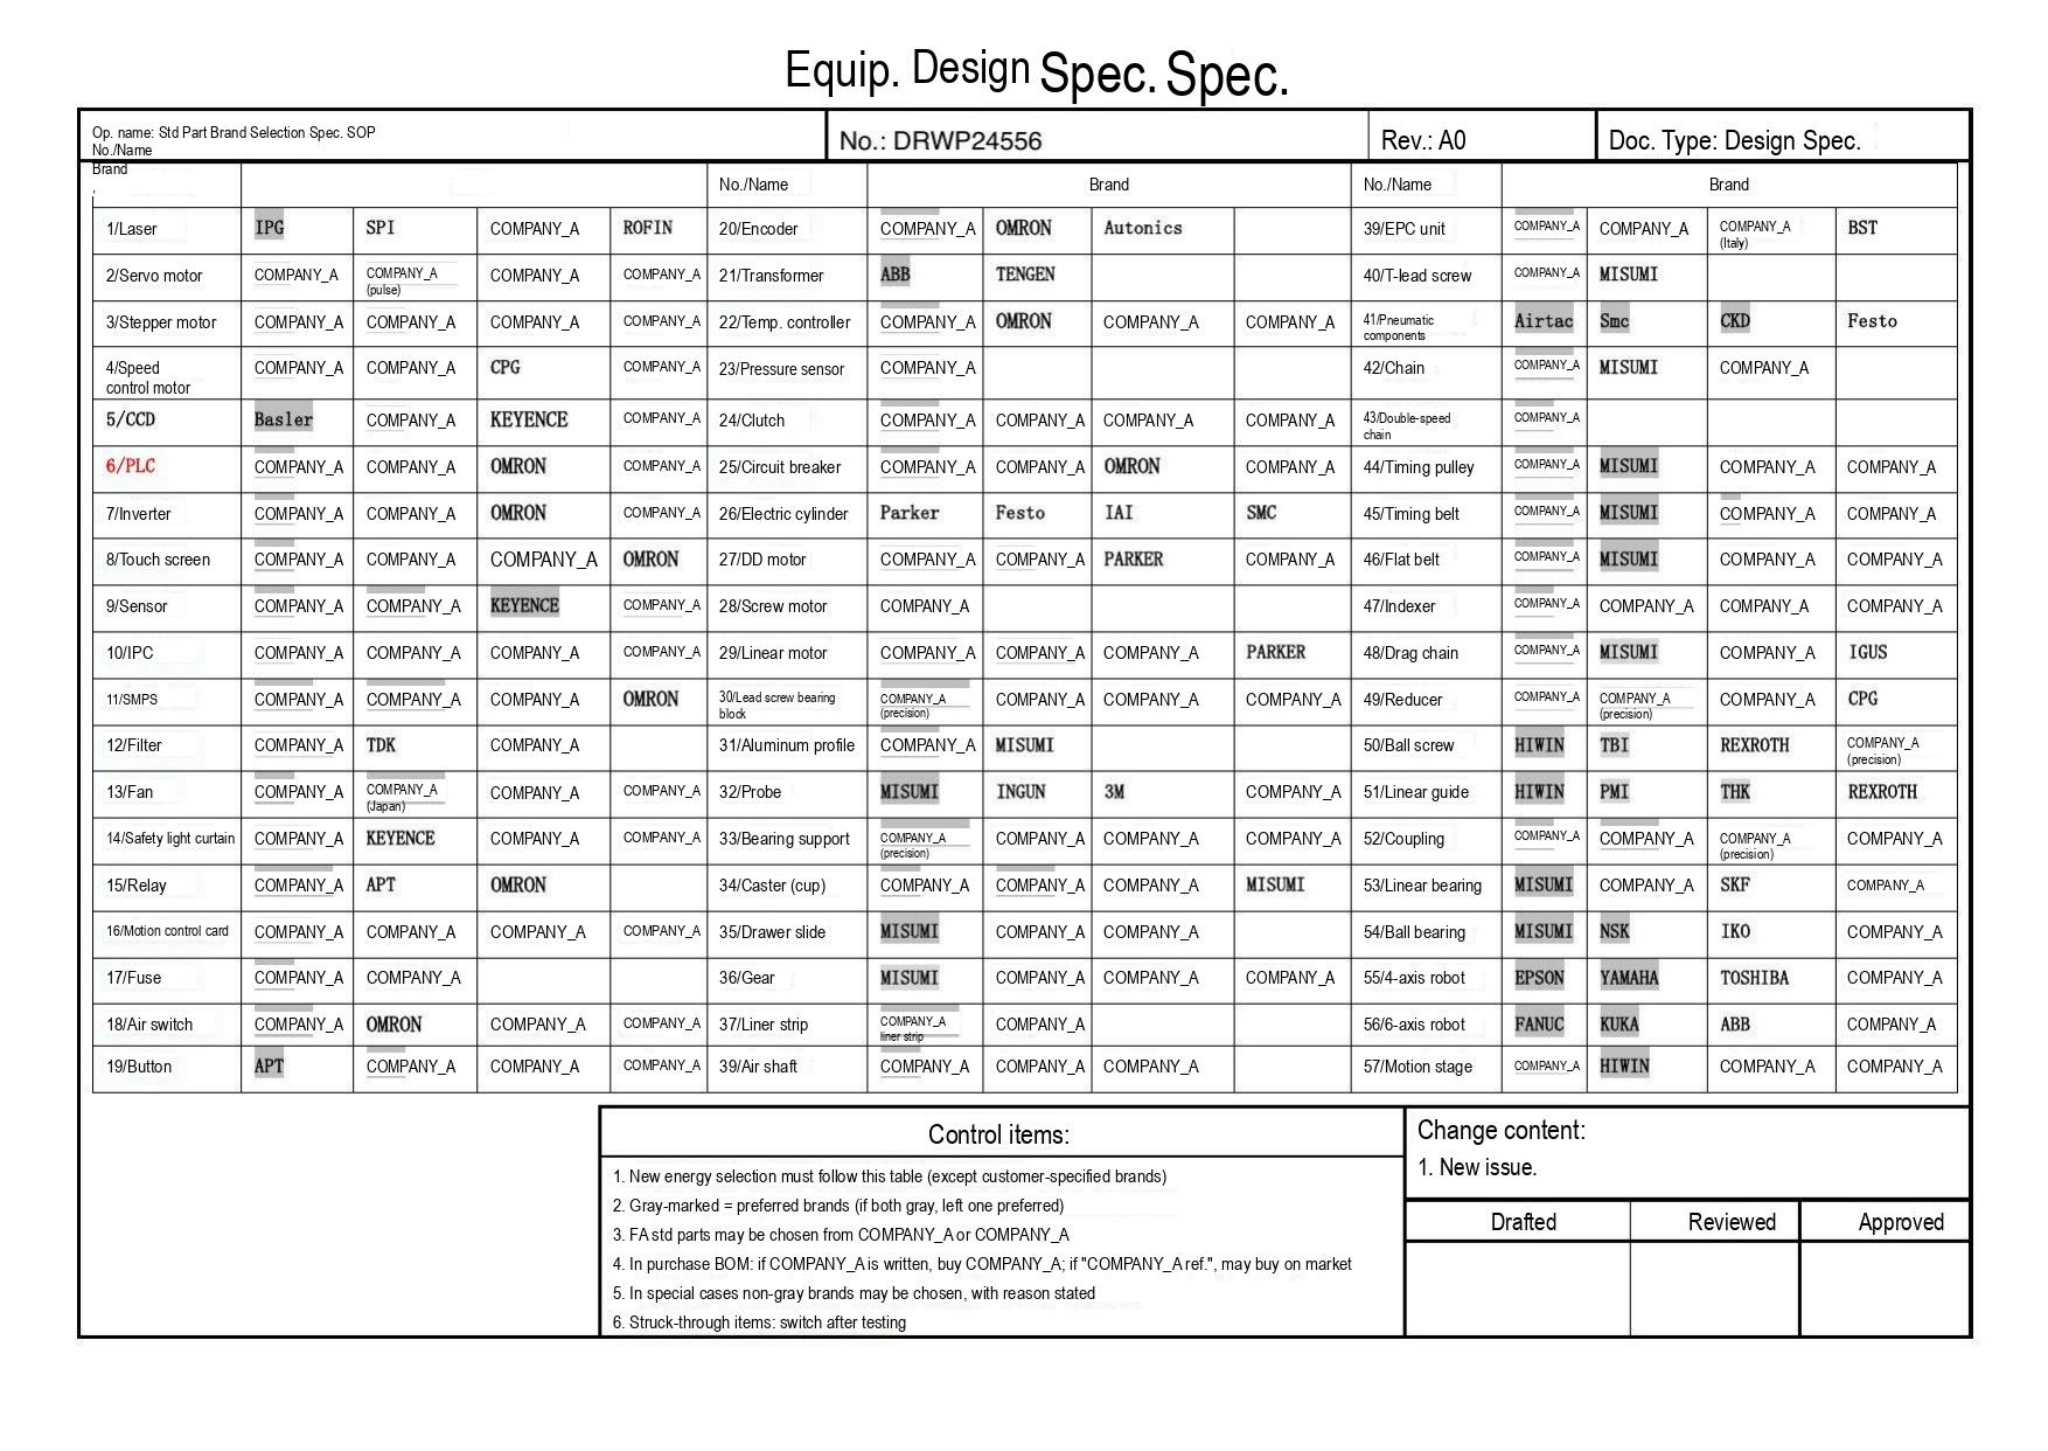Equip. Design Spec. Spec.

| Op. name: Std Part Brand Selection Spec. SOP | No.: DRWP24556 | Rev.: A0 | Doc. Type: Design Spec. |
|---|---|---|---|

| No./Name Brand | | | | | No./Name | Brand | | | | No./Name | Brand | | | |
|---|---|---|---|---|---|---|---|---|---|---|---|---|---|---|
| 1/Laser | IPG | SPI | COMPANY_A | ROFIN | 20/Encoder | COMPANY_A | OMRON | Autonics | | 39/EPC unit | COMPANY_A | COMPANY_A | COMPANY_A (Italy) | BST |
| 2/Servo motor | COMPANY_A | COMPANY_A (pulse) | COMPANY_A | COMPANY_A | 21/Transformer | ABB | TENGEN | | | 40/T-lead screw | COMPANY_A | MISUMI | | |
| 3/Stepper motor | COMPANY_A | COMPANY_A | COMPANY_A | COMPANY_A | 22/Temp. controller | COMPANY_A | OMRON | COMPANY_A | COMPANY_A | 41/Pneumatic components | Airtac | Smc | CKD | Festo |
| 4/Speed control motor | COMPANY_A | COMPANY_A | CPG | COMPANY_A | 23/Pressure sensor | COMPANY_A | | | | 42/Chain | COMPANY_A | MISUMI | COMPANY_A | |
| 5/CCD | Basler | COMPANY_A | KEYENCE | COMPANY_A | 24/Clutch | COMPANY_A | COMPANY_A | COMPANY_A | COMPANY_A | 43/Double-speed chain | COMPANY_A | | | |
| 6/PLC | COMPANY_A | COMPANY_A | OMRON | COMPANY_A | 25/Circuit breaker | COMPANY_A | COMPANY_A | OMRON | COMPANY_A | 44/Timing pulley | COMPANY_A | MISUMI | COMPANY_A | COMPANY_A |
| 7/Inverter | COMPANY_A | COMPANY_A | OMRON | COMPANY_A | 26/Electric cylinder | Parker | Festo | IAI | SMC | 45/Timing belt | COMPANY_A | MISUMI | COMPANY_A | COMPANY_A |
| 8/Touch screen | COMPANY_A | COMPANY_A | COMPANY_A | OMRON | 27/DD motor | COMPANY_A | COMPANY_A | PARKER | COMPANY_A | 46/Flat belt | COMPANY_A | MISUMI | COMPANY_A | COMPANY_A |
| 9/Sensor | COMPANY_A | COMPANY_A | KEYENCE | COMPANY_A | 28/Screw motor | COMPANY_A | | | | 47/Indexer | COMPANY_A | COMPANY_A | COMPANY_A | COMPANY_A |
| 10/IPC | COMPANY_A | COMPANY_A | COMPANY_A | COMPANY_A | 29/Linear motor | COMPANY_A | COMPANY_A | COMPANY_A | PARKER | 48/Drag chain | COMPANY_A | MISUMI | COMPANY_A | IGUS |
| 11/SMPS | COMPANY_A | COMPANY_A | COMPANY_A | OMRON | 30/Lead screw bearing block | COMPANY_A (precision) | COMPANY_A | COMPANY_A | COMPANY_A | 49/Reducer | COMPANY_A | COMPANY_A (precision) | COMPANY_A | CPG |
| 12/Filter | COMPANY_A | TDK | COMPANY_A | | 31/Aluminum profile | COMPANY_A | MISUMI | | | 50/Ball screw | HIWIN | TBI | REXROTH | COMPANY_A (precision) |
| 13/Fan | COMPANY_A | COMPANY_A (Japan) | COMPANY_A | COMPANY_A | 32/Probe | MISUMI | INGUN | 3M | COMPANY_A | 51/Linear guide | HIWIN | PMI | THK | REXROTH |
| 14/Safety light curtain | COMPANY_A | KEYENCE | COMPANY_A | COMPANY_A | 33/Bearing support | COMPANY_A (precision) | COMPANY_A | COMPANY_A | COMPANY_A | 52/Coupling | COMPANY_A | COMPANY_A | COMPANY_A (precision) | COMPANY_A |
| 15/Relay | COMPANY_A | APT | OMRON | | 34/Caster (cup) | COMPANY_A | COMPANY_A | COMPANY_A | MISUMI | 53/Linear bearing | MISUMI | COMPANY_A | SKF | COMPANY_A |
| 16/Motion control card | COMPANY_A | COMPANY_A | COMPANY_A | COMPANY_A | 35/Drawer slide | MISUMI | COMPANY_A | COMPANY_A | | 54/Ball bearing | MISUMI | NSK | IKO | COMPANY_A |
| 17/Fuse | COMPANY_A | COMPANY_A | | | 36/Gear | MISUMI | COMPANY_A | COMPANY_A | COMPANY_A | 55/4-axis robot | EPSON | YAMAHA | TOSHIBA | COMPANY_A |
| 18/Air switch | COMPANY_A | OMRON | COMPANY_A | COMPANY_A | 37/Liner strip | COMPANY_A liner strip | COMPANY_A | | | 56/6-axis robot | FANUC | KUKA | ABB | COMPANY_A |
| 19/Button | APT | COMPANY_A | COMPANY_A | COMPANY_A | 39/Air shaft | COMPANY_A | COMPANY_A | COMPANY_A | | 57/Motion stage | COMPANY_A | HIWIN | COMPANY_A | COMPANY_A |

Control items:
1. New energy selection must follow this table (except customer-specified brands)
2. Gray-marked = preferred brands (if both gray, left one preferred)
3. FA std parts may be chosen from COMPANY_A or COMPANY_A
4. In purchase BOM: if COMPANY_A is written, buy COMPANY_A; if "COMPANY_A ref.", may buy on market
5. In special cases non-gray brands may be chosen, with reason stated
6. Struck-through items: switch after testing

Change content:
1. New issue.

| Drafted | Reviewed | Approved |
|---|---|---|
| | | |